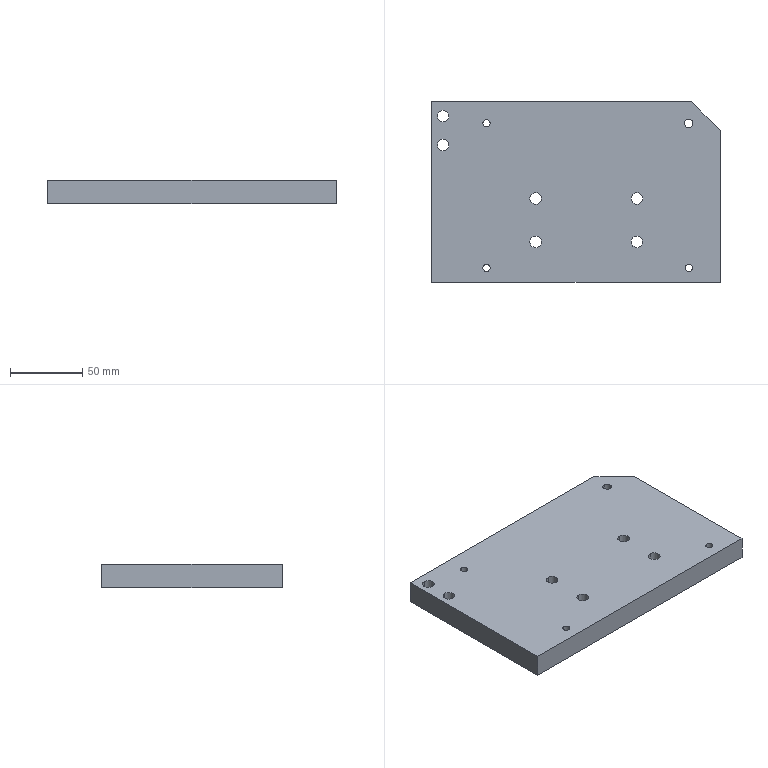Part | STEP file | [15] | 1 solid | 27 faces | box 200 x 125 x 16 mm | volume 390580 mm3 | cylinder 20 | plane 7 | commonest cylinder face diameters 8 x12 5 x6 6 x2
STEP:
#1=CARTESIAN_POINT('',(175.,113.,0.));
#2=VERTEX_POINT('',#1);
#3=CARTESIAN_POINT('',(175.,107.,0.));
#4=VERTEX_POINT('',#3);
#5=CARTESIAN_POINT('',(175.,110.,0.));
#6=DIRECTION('',(0.,0.,1.));
#7=DIRECTION('',(0.,-1.,0.));
#8=AXIS2_PLACEMENT_3D('',#5,#6,#7);
#9=CIRCLE('',#8,3.);
#10=EDGE_CURVE('',#2,#4,#9,.T.);
#11=ORIENTED_EDGE('',*,*,#10,.F.);
#12=CARTESIAN_POINT('',(175.,113.,16.));
#13=VERTEX_POINT('',#12);
#14=CARTESIAN_POINT('',(175.,113.,0.));
#15=DIRECTION('',(0.,0.,1.));
#16=VECTOR('',#15,1000.);
#17=LINE('',#14,#16);
#18=EDGE_CURVE('',#2,#13,#17,.T.);
#19=ORIENTED_EDGE('',*,*,#18,.T.);
#20=CARTESIAN_POINT('',(175.,107.,16.));
#21=VERTEX_POINT('',#20);
#22=CARTESIAN_POINT('',(175.,110.,16.));
#23=DIRECTION('',(0.,0.,-1.));
#24=DIRECTION('',(0.,1.,0.));
#25=AXIS2_PLACEMENT_3D('',#22,#23,#24);
#26=CIRCLE('',#25,3.);
#27=EDGE_CURVE('',#21,#13,#26,.T.);
#28=ORIENTED_EDGE('',*,*,#27,.F.);
#29=CARTESIAN_POINT('',(175.,107.,0.));
#30=DIRECTION('',(0.,0.,1.));
#31=VECTOR('',#30,1000.);
#32=LINE('',#29,#31);
#33=EDGE_CURVE('',#4,#21,#32,.T.);
#34=ORIENTED_EDGE('',*,*,#33,.F.);
#35=EDGE_LOOP('',(#11,#19,#28,#34));
#36=FACE_OUTER_BOUND('',#35,.T.);
#37=CARTESIAN_POINT('',(175.,110.,0.));
#38=DIRECTION('',(0.,0.,1.));
#39=DIRECTION('',(0.,-1.,0.));
#40=AXIS2_PLACEMENT_3D('',#37,#38,#39);
#41=CYLINDRICAL_SURFACE('',#40,3.);
#42=ADVANCED_FACE('',(#36),#41,.F.);
#43=CARTESIAN_POINT('',(35.,112.5,0.));
#44=VERTEX_POINT('',#43);
#45=CARTESIAN_POINT('',(35.,107.5,0.));
#46=VERTEX_POINT('',#45);
#47=CARTESIAN_POINT('',(35.,110.,0.));
#48=DIRECTION('',(0.,0.,1.));
#49=DIRECTION('',(0.,-1.,0.));
#50=AXIS2_PLACEMENT_3D('',#47,#48,#49);
#51=CIRCLE('',#50,2.5);
#52=EDGE_CURVE('',#44,#46,#51,.T.);
#53=ORIENTED_EDGE('',*,*,#52,.F.);
#54=CARTESIAN_POINT('',(35.,112.5,16.));
#55=VERTEX_POINT('',#54);
#56=CARTESIAN_POINT('',(35.,112.5,0.));
#57=DIRECTION('',(0.,0.,1.));
#58=VECTOR('',#57,1000.);
#59=LINE('',#56,#58);
#60=EDGE_CURVE('',#44,#55,#59,.T.);
#61=ORIENTED_EDGE('',*,*,#60,.T.);
#62=CARTESIAN_POINT('',(35.,107.5,16.));
#63=VERTEX_POINT('',#62);
#64=CARTESIAN_POINT('',(35.,110.,16.));
#65=DIRECTION('',(0.,0.,-1.));
#66=DIRECTION('',(0.,1.,0.));
#67=AXIS2_PLACEMENT_3D('',#64,#65,#66);
#68=CIRCLE('',#67,2.5);
#69=EDGE_CURVE('',#63,#55,#68,.T.);
#70=ORIENTED_EDGE('',*,*,#69,.F.);
#71=CARTESIAN_POINT('',(35.,107.5,0.));
#72=DIRECTION('',(0.,0.,1.));
#73=VECTOR('',#72,1000.);
#74=LINE('',#71,#73);
#75=EDGE_CURVE('',#46,#63,#74,.T.);
#76=ORIENTED_EDGE('',*,*,#75,.F.);
#77=EDGE_LOOP('',(#53,#61,#70,#76));
#78=FACE_OUTER_BOUND('',#77,.T.);
#79=CARTESIAN_POINT('',(35.,110.,0.));
#80=DIRECTION('',(0.,0.,1.));
#81=DIRECTION('',(0.,-1.,0.));
#82=AXIS2_PLACEMENT_3D('',#79,#80,#81);
#83=CYLINDRICAL_SURFACE('',#82,2.5);
#84=ADVANCED_FACE('',(#78),#83,.F.);
#85=CARTESIAN_POINT('',(175.,12.5,0.));
#86=VERTEX_POINT('',#85);
#87=CARTESIAN_POINT('',(175.,7.5,0.));
#88=VERTEX_POINT('',#87);
#89=CARTESIAN_POINT('',(175.,10.,0.));
#90=DIRECTION('',(0.,0.,1.));
#91=DIRECTION('',(0.,-1.,0.));
#92=AXIS2_PLACEMENT_3D('',#89,#90,#91);
#93=CIRCLE('',#92,2.5);
#94=EDGE_CURVE('',#86,#88,#93,.T.);
#95=ORIENTED_EDGE('',*,*,#94,.F.);
#96=CARTESIAN_POINT('',(175.,12.5,16.));
#97=VERTEX_POINT('',#96);
#98=CARTESIAN_POINT('',(175.,12.5,0.));
#99=DIRECTION('',(0.,0.,1.));
#100=VECTOR('',#99,1000.);
#101=LINE('',#98,#100);
#102=EDGE_CURVE('',#86,#97,#101,.T.);
#103=ORIENTED_EDGE('',*,*,#102,.T.);
#104=CARTESIAN_POINT('',(175.,7.5,16.));
#105=VERTEX_POINT('',#104);
#106=CARTESIAN_POINT('',(175.,10.,16.));
#107=DIRECTION('',(0.,0.,-1.));
#108=DIRECTION('',(0.,1.,0.));
#109=AXIS2_PLACEMENT_3D('',#106,#107,#108);
#110=CIRCLE('',#109,2.5);
#111=EDGE_CURVE('',#105,#97,#110,.T.);
#112=ORIENTED_EDGE('',*,*,#111,.F.);
#113=CARTESIAN_POINT('',(175.,7.5,0.));
#114=DIRECTION('',(0.,0.,1.));
#115=VECTOR('',#114,1000.);
#116=LINE('',#113,#115);
#117=EDGE_CURVE('',#88,#105,#116,.T.);
#118=ORIENTED_EDGE('',*,*,#117,.F.);
#119=EDGE_LOOP('',(#95,#103,#112,#118));
#120=FACE_OUTER_BOUND('',#119,.T.);
#121=CARTESIAN_POINT('',(175.,10.,0.));
#122=DIRECTION('',(0.,0.,1.));
#123=DIRECTION('',(0.,-1.,0.));
#124=AXIS2_PLACEMENT_3D('',#121,#122,#123);
#125=CYLINDRICAL_SURFACE('',#124,2.5);
#126=ADVANCED_FACE('',(#120),#125,.F.);
#127=CARTESIAN_POINT('',(35.,12.5,0.));
#128=VERTEX_POINT('',#127);
#129=CARTESIAN_POINT('',(35.,7.5,0.));
#130=VERTEX_POINT('',#129);
#131=CARTESIAN_POINT('',(35.,10.,0.));
#132=DIRECTION('',(0.,0.,1.));
#133=DIRECTION('',(0.,-1.,0.));
#134=AXIS2_PLACEMENT_3D('',#131,#132,#133);
#135=CIRCLE('',#134,2.5);
#136=EDGE_CURVE('',#128,#130,#135,.T.);
#137=ORIENTED_EDGE('',*,*,#136,.F.);
#138=CARTESIAN_POINT('',(35.,12.5,16.));
#139=VERTEX_POINT('',#138);
#140=CARTESIAN_POINT('',(35.,12.5,0.));
#141=DIRECTION('',(0.,0.,1.));
#142=VECTOR('',#141,1000.);
#143=LINE('',#140,#142);
#144=EDGE_CURVE('',#128,#139,#143,.T.);
#145=ORIENTED_EDGE('',*,*,#144,.T.);
#146=CARTESIAN_POINT('',(35.,7.5,16.));
#147=VERTEX_POINT('',#146);
#148=CARTESIAN_POINT('',(35.,10.,16.));
#149=DIRECTION('',(0.,0.,-1.));
#150=DIRECTION('',(0.,1.,0.));
#151=AXIS2_PLACEMENT_3D('',#148,#149,#150);
#152=CIRCLE('',#151,2.5);
#153=EDGE_CURVE('',#147,#139,#152,.T.);
#154=ORIENTED_EDGE('',*,*,#153,.F.);
#155=CARTESIAN_POINT('',(35.,7.5,0.));
#156=DIRECTION('',(0.,0.,1.));
#157=VECTOR('',#156,1000.);
#158=LINE('',#155,#157);
#159=EDGE_CURVE('',#130,#147,#158,.T.);
#160=ORIENTED_EDGE('',*,*,#159,.F.);
#161=EDGE_LOOP('',(#137,#145,#154,#160));
#162=FACE_OUTER_BOUND('',#161,.T.);
#163=CARTESIAN_POINT('',(35.,10.,0.));
#164=DIRECTION('',(0.,0.,1.));
#165=DIRECTION('',(0.,-1.,0.));
#166=AXIS2_PLACEMENT_3D('',#163,#164,#165);
#167=CYLINDRICAL_SURFACE('',#166,2.5);
#168=ADVANCED_FACE('',(#162),#167,.F.);
#169=CARTESIAN_POINT('',(5.,119.,0.));
#170=VERTEX_POINT('',#169);
#171=CARTESIAN_POINT('',(5.,111.,0.));
#172=VERTEX_POINT('',#171);
#173=CARTESIAN_POINT('',(5.,115.,0.));
#174=DIRECTION('',(0.,0.,1.));
#175=DIRECTION('',(0.,-1.,0.));
#176=AXIS2_PLACEMENT_3D('',#173,#174,#175);
#177=CIRCLE('',#176,4.);
#178=EDGE_CURVE('',#170,#172,#177,.T.);
#179=ORIENTED_EDGE('',*,*,#178,.F.);
#180=CARTESIAN_POINT('',(5.,119.,16.));
#181=VERTEX_POINT('',#180);
#182=CARTESIAN_POINT('',(5.,119.,0.));
#183=DIRECTION('',(0.,0.,1.));
#184=VECTOR('',#183,1000.);
#185=LINE('',#182,#184);
#186=EDGE_CURVE('',#170,#181,#185,.T.);
#187=ORIENTED_EDGE('',*,*,#186,.T.);
#188=CARTESIAN_POINT('',(5.,111.,16.));
#189=VERTEX_POINT('',#188);
#190=CARTESIAN_POINT('',(5.,115.,16.));
#191=DIRECTION('',(0.,0.,-1.));
#192=DIRECTION('',(0.,1.,0.));
#193=AXIS2_PLACEMENT_3D('',#190,#191,#192);
#194=CIRCLE('',#193,4.);
#195=EDGE_CURVE('',#189,#181,#194,.T.);
#196=ORIENTED_EDGE('',*,*,#195,.F.);
#197=CARTESIAN_POINT('',(5.,111.,0.));
#198=DIRECTION('',(0.,0.,1.));
#199=VECTOR('',#198,1000.);
#200=LINE('',#197,#199);
#201=EDGE_CURVE('',#172,#189,#200,.T.);
#202=ORIENTED_EDGE('',*,*,#201,.F.);
#203=EDGE_LOOP('',(#179,#187,#196,#202));
#204=FACE_OUTER_BOUND('',#203,.T.);
#205=CARTESIAN_POINT('',(5.,115.,0.));
#206=DIRECTION('',(0.,0.,1.));
#207=DIRECTION('',(0.,-1.,0.));
#208=AXIS2_PLACEMENT_3D('',#205,#206,#207);
#209=CYLINDRICAL_SURFACE('',#208,4.);
#210=ADVANCED_FACE('',(#204),#209,.F.);
#211=CARTESIAN_POINT('',(5.,99.,0.));
#212=VERTEX_POINT('',#211);
#213=CARTESIAN_POINT('',(5.,91.,0.));
#214=VERTEX_POINT('',#213);
#215=CARTESIAN_POINT('',(5.,95.,0.));
#216=DIRECTION('',(0.,0.,1.));
#217=DIRECTION('',(0.,-1.,0.));
#218=AXIS2_PLACEMENT_3D('',#215,#216,#217);
#219=CIRCLE('',#218,4.);
#220=EDGE_CURVE('',#212,#214,#219,.T.);
#221=ORIENTED_EDGE('',*,*,#220,.F.);
#222=CARTESIAN_POINT('',(5.,99.,16.));
#223=VERTEX_POINT('',#222);
#224=CARTESIAN_POINT('',(5.,99.,0.));
#225=DIRECTION('',(0.,0.,1.));
#226=VECTOR('',#225,1000.);
#227=LINE('',#224,#226);
#228=EDGE_CURVE('',#212,#223,#227,.T.);
#229=ORIENTED_EDGE('',*,*,#228,.T.);
#230=CARTESIAN_POINT('',(5.,91.,16.));
#231=VERTEX_POINT('',#230);
#232=CARTESIAN_POINT('',(5.,95.,16.));
#233=DIRECTION('',(0.,0.,-1.));
#234=DIRECTION('',(0.,1.,0.));
#235=AXIS2_PLACEMENT_3D('',#232,#233,#234);
#236=CIRCLE('',#235,4.);
#237=EDGE_CURVE('',#231,#223,#236,.T.);
#238=ORIENTED_EDGE('',*,*,#237,.F.);
#239=CARTESIAN_POINT('',(5.,91.,0.));
#240=DIRECTION('',(0.,0.,1.));
#241=VECTOR('',#240,1000.);
#242=LINE('',#239,#241);
#243=EDGE_CURVE('',#214,#231,#242,.T.);
#244=ORIENTED_EDGE('',*,*,#243,.F.);
#245=EDGE_LOOP('',(#221,#229,#238,#244));
#246=FACE_OUTER_BOUND('',#245,.T.);
#247=CARTESIAN_POINT('',(5.,95.,0.));
#248=DIRECTION('',(0.,0.,1.));
#249=DIRECTION('',(0.,-1.,0.));
#250=AXIS2_PLACEMENT_3D('',#247,#248,#249);
#251=CYLINDRICAL_SURFACE('',#250,4.);
#252=ADVANCED_FACE('',(#246),#251,.F.);
#253=CARTESIAN_POINT('',(139.1,32.,0.));
#254=VERTEX_POINT('',#253);
#255=CARTESIAN_POINT('',(139.1,24.,0.));
#256=VERTEX_POINT('',#255);
#257=CARTESIAN_POINT('',(139.1,28.,0.));
#258=DIRECTION('',(0.,0.,1.));
#259=DIRECTION('',(0.,-1.,0.));
#260=AXIS2_PLACEMENT_3D('',#257,#258,#259);
#261=CIRCLE('',#260,4.);
#262=EDGE_CURVE('',#254,#256,#261,.T.);
#263=ORIENTED_EDGE('',*,*,#262,.F.);
#264=CARTESIAN_POINT('',(139.1,32.,16.));
#265=VERTEX_POINT('',#264);
#266=CARTESIAN_POINT('',(139.1,32.,0.));
#267=DIRECTION('',(0.,0.,1.));
#268=VECTOR('',#267,1000.);
#269=LINE('',#266,#268);
#270=EDGE_CURVE('',#254,#265,#269,.T.);
#271=ORIENTED_EDGE('',*,*,#270,.T.);
#272=CARTESIAN_POINT('',(139.1,24.,16.));
#273=VERTEX_POINT('',#272);
#274=CARTESIAN_POINT('',(139.1,28.,16.));
#275=DIRECTION('',(0.,0.,-1.));
#276=DIRECTION('',(0.,1.,0.));
#277=AXIS2_PLACEMENT_3D('',#274,#275,#276);
#278=CIRCLE('',#277,4.);
#279=EDGE_CURVE('',#273,#265,#278,.T.);
#280=ORIENTED_EDGE('',*,*,#279,.F.);
#281=CARTESIAN_POINT('',(139.1,24.,0.));
#282=DIRECTION('',(0.,0.,1.));
#283=VECTOR('',#282,1000.);
#284=LINE('',#281,#283);
#285=EDGE_CURVE('',#256,#273,#284,.T.);
#286=ORIENTED_EDGE('',*,*,#285,.F.);
#287=EDGE_LOOP('',(#263,#271,#280,#286));
#288=FACE_OUTER_BOUND('',#287,.T.);
#289=CARTESIAN_POINT('',(139.1,28.,0.));
#290=DIRECTION('',(0.,0.,1.));
#291=DIRECTION('',(0.,-1.,0.));
#292=AXIS2_PLACEMENT_3D('',#289,#290,#291);
#293=CYLINDRICAL_SURFACE('',#292,4.);
#294=ADVANCED_FACE('',(#288),#293,.F.);
#295=CARTESIAN_POINT('',(139.1,62.,0.));
#296=VERTEX_POINT('',#295);
#297=CARTESIAN_POINT('',(139.1,54.,0.));
#298=VERTEX_POINT('',#297);
#299=CARTESIAN_POINT('',(139.1,58.,0.));
#300=DIRECTION('',(0.,0.,1.));
#301=DIRECTION('',(0.,-1.,0.));
#302=AXIS2_PLACEMENT_3D('',#299,#300,#301);
#303=CIRCLE('',#302,4.);
#304=EDGE_CURVE('',#296,#298,#303,.T.);
#305=ORIENTED_EDGE('',*,*,#304,.F.);
#306=CARTESIAN_POINT('',(139.1,62.,16.));
#307=VERTEX_POINT('',#306);
#308=CARTESIAN_POINT('',(139.1,62.,0.));
#309=DIRECTION('',(0.,0.,1.));
#310=VECTOR('',#309,1000.);
#311=LINE('',#308,#310);
#312=EDGE_CURVE('',#296,#307,#311,.T.);
#313=ORIENTED_EDGE('',*,*,#312,.T.);
#314=CARTESIAN_POINT('',(139.1,54.,16.));
#315=VERTEX_POINT('',#314);
#316=CARTESIAN_POINT('',(139.1,58.,16.));
#317=DIRECTION('',(0.,0.,-1.));
#318=DIRECTION('',(0.,1.,0.));
#319=AXIS2_PLACEMENT_3D('',#316,#317,#318);
#320=CIRCLE('',#319,4.);
#321=EDGE_CURVE('',#315,#307,#320,.T.);
#322=ORIENTED_EDGE('',*,*,#321,.F.);
#323=CARTESIAN_POINT('',(139.1,54.,0.));
#324=DIRECTION('',(0.,0.,1.));
#325=VECTOR('',#324,1000.);
#326=LINE('',#323,#325);
#327=EDGE_CURVE('',#298,#315,#326,.T.);
#328=ORIENTED_EDGE('',*,*,#327,.F.);
#329=EDGE_LOOP('',(#305,#313,#322,#328));
#330=FACE_OUTER_BOUND('',#329,.T.);
#331=CARTESIAN_POINT('',(139.1,58.,0.));
#332=DIRECTION('',(0.,0.,1.));
#333=DIRECTION('',(0.,-1.,0.));
#334=AXIS2_PLACEMENT_3D('',#331,#332,#333);
#335=CYLINDRICAL_SURFACE('',#334,4.);
#336=ADVANCED_FACE('',(#330),#335,.F.);
#337=CARTESIAN_POINT('',(69.1,32.,0.));
#338=VERTEX_POINT('',#337);
#339=CARTESIAN_POINT('',(69.1,24.,0.));
#340=VERTEX_POINT('',#339);
#341=CARTESIAN_POINT('',(69.1,28.,0.));
#342=DIRECTION('',(0.,0.,1.));
#343=DIRECTION('',(0.,-1.,0.));
#344=AXIS2_PLACEMENT_3D('',#341,#342,#343);
#345=CIRCLE('',#344,4.);
#346=EDGE_CURVE('',#338,#340,#345,.T.);
#347=ORIENTED_EDGE('',*,*,#346,.F.);
#348=CARTESIAN_POINT('',(69.1,32.,16.));
#349=VERTEX_POINT('',#348);
#350=CARTESIAN_POINT('',(69.1,32.,0.));
#351=DIRECTION('',(0.,0.,1.));
#352=VECTOR('',#351,1000.);
#353=LINE('',#350,#352);
#354=EDGE_CURVE('',#338,#349,#353,.T.);
#355=ORIENTED_EDGE('',*,*,#354,.T.);
#356=CARTESIAN_POINT('',(69.1,24.,16.));
#357=VERTEX_POINT('',#356);
#358=CARTESIAN_POINT('',(69.1,28.,16.));
#359=DIRECTION('',(0.,0.,-1.));
#360=DIRECTION('',(0.,1.,0.));
#361=AXIS2_PLACEMENT_3D('',#358,#359,#360);
#362=CIRCLE('',#361,4.);
#363=EDGE_CURVE('',#357,#349,#362,.T.);
#364=ORIENTED_EDGE('',*,*,#363,.F.);
#365=CARTESIAN_POINT('',(69.1,24.,0.));
#366=DIRECTION('',(0.,0.,1.));
#367=VECTOR('',#366,1000.);
#368=LINE('',#365,#367);
#369=EDGE_CURVE('',#340,#357,#368,.T.);
#370=ORIENTED_EDGE('',*,*,#369,.F.);
#371=EDGE_LOOP('',(#347,#355,#364,#370));
#372=FACE_OUTER_BOUND('',#371,.T.);
#373=CARTESIAN_POINT('',(69.1,28.,0.));
#374=DIRECTION('',(0.,0.,1.));
#375=DIRECTION('',(0.,-1.,0.));
#376=AXIS2_PLACEMENT_3D('',#373,#374,#375);
#377=CYLINDRICAL_SURFACE('',#376,4.);
#378=ADVANCED_FACE('',(#372),#377,.F.);
#379=CARTESIAN_POINT('',(69.1,62.,0.));
#380=VERTEX_POINT('',#379);
#381=CARTESIAN_POINT('',(69.1,54.,0.));
#382=VERTEX_POINT('',#381);
#383=CARTESIAN_POINT('',(69.1,58.,0.));
#384=DIRECTION('',(0.,0.,1.));
#385=DIRECTION('',(0.,-1.,0.));
#386=AXIS2_PLACEMENT_3D('',#383,#384,#385);
#387=CIRCLE('',#386,4.);
#388=EDGE_CURVE('',#380,#382,#387,.T.);
#389=ORIENTED_EDGE('',*,*,#388,.F.);
#390=CARTESIAN_POINT('',(69.1,62.,16.));
#391=VERTEX_POINT('',#390);
#392=CARTESIAN_POINT('',(69.1,62.,0.));
#393=DIRECTION('',(0.,0.,1.));
#394=VECTOR('',#393,1000.);
#395=LINE('',#392,#394);
#396=EDGE_CURVE('',#380,#391,#395,.T.);
#397=ORIENTED_EDGE('',*,*,#396,.T.);
#398=CARTESIAN_POINT('',(69.1,54.,16.));
#399=VERTEX_POINT('',#398);
#400=CARTESIAN_POINT('',(69.1,58.,16.));
#401=DIRECTION('',(0.,0.,-1.));
#402=DIRECTION('',(0.,1.,0.));
#403=AXIS2_PLACEMENT_3D('',#400,#401,#402);
#404=CIRCLE('',#403,4.);
#405=EDGE_CURVE('',#399,#391,#404,.T.);
#406=ORIENTED_EDGE('',*,*,#405,.F.);
#407=CARTESIAN_POINT('',(69.1,54.,0.));
#408=DIRECTION('',(0.,0.,1.));
#409=VECTOR('',#408,1000.);
#410=LINE('',#407,#409);
#411=EDGE_CURVE('',#382,#399,#410,.T.);
#412=ORIENTED_EDGE('',*,*,#411,.F.);
#413=EDGE_LOOP('',(#389,#397,#406,#412));
#414=FACE_OUTER_BOUND('',#413,.T.);
#415=CARTESIAN_POINT('',(69.1,58.,0.));
#416=DIRECTION('',(0.,0.,1.));
#417=DIRECTION('',(0.,-1.,0.));
#418=AXIS2_PLACEMENT_3D('',#415,#416,#417);
#419=CYLINDRICAL_SURFACE('',#418,4.);
#420=ADVANCED_FACE('',(#414),#419,.F.);
#421=CARTESIAN_POINT('',(175.,110.,0.));
#422=DIRECTION('',(0.,0.,1.));
#423=DIRECTION('',(0.,-1.,0.));
#424=AXIS2_PLACEMENT_3D('',#421,#422,#423);
#425=CIRCLE('',#424,3.);
#426=EDGE_CURVE('',#4,#2,#425,.T.);
#427=ORIENTED_EDGE('',*,*,#426,.T.);
#428=ORIENTED_EDGE('',*,*,#10,.T.);
#429=EDGE_LOOP('',(#427,#428));
#430=FACE_BOUND('',#429,.T.);
#431=CARTESIAN_POINT('',(35.,110.,0.));
#432=DIRECTION('',(0.,0.,1.));
#433=DIRECTION('',(0.,-1.,0.));
#434=AXIS2_PLACEMENT_3D('',#431,#432,#433);
#435=CIRCLE('',#434,2.5);
#436=EDGE_CURVE('',#46,#44,#435,.T.);
#437=ORIENTED_EDGE('',*,*,#436,.T.);
#438=ORIENTED_EDGE('',*,*,#52,.T.);
#439=EDGE_LOOP('',(#437,#438));
#440=FACE_BOUND('',#439,.T.);
#441=CARTESIAN_POINT('',(175.,10.,0.));
#442=DIRECTION('',(0.,0.,1.));
#443=DIRECTION('',(0.,-1.,0.));
#444=AXIS2_PLACEMENT_3D('',#441,#442,#443);
#445=CIRCLE('',#444,2.5);
#446=EDGE_CURVE('',#88,#86,#445,.T.);
#447=ORIENTED_EDGE('',*,*,#446,.T.);
#448=ORIENTED_EDGE('',*,*,#94,.T.);
#449=EDGE_LOOP('',(#447,#448));
#450=FACE_BOUND('',#449,.T.);
#451=CARTESIAN_POINT('',(35.,10.,0.));
#452=DIRECTION('',(0.,0.,1.));
#453=DIRECTION('',(0.,-1.,0.));
#454=AXIS2_PLACEMENT_3D('',#451,#452,#453);
#455=CIRCLE('',#454,2.5);
#456=EDGE_CURVE('',#130,#128,#455,.T.);
#457=ORIENTED_EDGE('',*,*,#456,.T.);
#458=ORIENTED_EDGE('',*,*,#136,.T.);
#459=EDGE_LOOP('',(#457,#458));
#460=FACE_BOUND('',#459,.T.);
#461=CARTESIAN_POINT('',(5.,115.,0.));
#462=DIRECTION('',(0.,0.,1.));
#463=DIRECTION('',(0.,-1.,0.));
#464=AXIS2_PLACEMENT_3D('',#461,#462,#463);
#465=CIRCLE('',#464,4.);
#466=EDGE_CURVE('',#172,#170,#465,.T.);
#467=ORIENTED_EDGE('',*,*,#466,.T.);
#468=ORIENTED_EDGE('',*,*,#178,.T.);
#469=EDGE_LOOP('',(#467,#468));
#470=FACE_BOUND('',#469,.T.);
#471=CARTESIAN_POINT('',(5.,95.,0.));
#472=DIRECTION('',(0.,0.,1.));
#473=DIRECTION('',(0.,-1.,0.));
#474=AXIS2_PLACEMENT_3D('',#471,#472,#473);
#475=CIRCLE('',#474,4.);
#476=EDGE_CURVE('',#214,#212,#475,.T.);
#477=ORIENTED_EDGE('',*,*,#476,.T.);
#478=ORIENTED_EDGE('',*,*,#220,.T.);
#479=EDGE_LOOP('',(#477,#478));
#480=FACE_BOUND('',#479,.T.);
#481=CARTESIAN_POINT('',(139.1,28.,0.));
#482=DIRECTION('',(0.,0.,1.));
#483=DIRECTION('',(0.,-1.,0.));
#484=AXIS2_PLACEMENT_3D('',#481,#482,#483);
#485=CIRCLE('',#484,4.);
#486=EDGE_CURVE('',#256,#254,#485,.T.);
#487=ORIENTED_EDGE('',*,*,#486,.T.);
#488=ORIENTED_EDGE('',*,*,#262,.T.);
#489=EDGE_LOOP('',(#487,#488));
#490=FACE_BOUND('',#489,.T.);
#491=CARTESIAN_POINT('',(139.1,58.,0.));
#492=DIRECTION('',(0.,0.,1.));
#493=DIRECTION('',(0.,-1.,0.));
#494=AXIS2_PLACEMENT_3D('',#491,#492,#493);
#495=CIRCLE('',#494,4.);
#496=EDGE_CURVE('',#298,#296,#495,.T.);
#497=ORIENTED_EDGE('',*,*,#496,.T.);
#498=ORIENTED_EDGE('',*,*,#304,.T.);
#499=EDGE_LOOP('',(#497,#498));
#500=FACE_BOUND('',#499,.T.);
#501=CARTESIAN_POINT('',(69.1,28.,0.));
#502=DIRECTION('',(0.,0.,1.));
#503=DIRECTION('',(0.,-1.,0.));
#504=AXIS2_PLACEMENT_3D('',#501,#502,#503);
#505=CIRCLE('',#504,4.);
#506=EDGE_CURVE('',#340,#338,#505,.T.);
#507=ORIENTED_EDGE('',*,*,#506,.T.);
#508=ORIENTED_EDGE('',*,*,#346,.T.);
#509=EDGE_LOOP('',(#507,#508));
#510=FACE_BOUND('',#509,.T.);
#511=CARTESIAN_POINT('',(69.1,58.,0.));
#512=DIRECTION('',(0.,0.,1.));
#513=DIRECTION('',(0.,-1.,0.));
#514=AXIS2_PLACEMENT_3D('',#511,#512,#513);
#515=CIRCLE('',#514,4.);
#516=EDGE_CURVE('',#382,#380,#515,.T.);
#517=ORIENTED_EDGE('',*,*,#516,.T.);
#518=ORIENTED_EDGE('',*,*,#388,.T.);
#519=EDGE_LOOP('',(#517,#518));
#520=FACE_BOUND('',#519,.T.);
#521=CARTESIAN_POINT('',(177.,125.,0.));
#522=VERTEX_POINT('',#521);
#523=CARTESIAN_POINT('',(-3.,125.,0.));
#524=VERTEX_POINT('',#523);
#525=CARTESIAN_POINT('',(97.,125.,0.));
#526=DIRECTION('',(-1.,0.,0.));
#527=VECTOR('',#526,1000.);
#528=LINE('',#525,#527);
#529=EDGE_CURVE('',#522,#524,#528,.T.);
#530=ORIENTED_EDGE('',*,*,#529,.F.);
#531=CARTESIAN_POINT('',(197.,105.,0.));
#532=VERTEX_POINT('',#531);
#533=CARTESIAN_POINT('',(168.25,133.75,0.));
#534=DIRECTION('',(0.7071,-0.7071,0.));
#535=VECTOR('',#534,1000.);
#536=LINE('',#533,#535);
#537=EDGE_CURVE('',#522,#532,#536,.T.);
#538=ORIENTED_EDGE('',*,*,#537,.T.);
#539=CARTESIAN_POINT('',(197.,0.,0.));
#540=VERTEX_POINT('',#539);
#541=CARTESIAN_POINT('',(197.,62.5,0.));
#542=DIRECTION('',(0.,1.,0.));
#543=VECTOR('',#542,1000.);
#544=LINE('',#541,#543);
#545=EDGE_CURVE('',#540,#532,#544,.T.);
#546=ORIENTED_EDGE('',*,*,#545,.F.);
#547=CARTESIAN_POINT('',(-3.,0.,0.));
#548=VERTEX_POINT('',#547);
#549=CARTESIAN_POINT('',(97.,0.,0.));
#550=DIRECTION('',(1.,0.,0.));
#551=VECTOR('',#550,1000.);
#552=LINE('',#549,#551);
#553=EDGE_CURVE('',#548,#540,#552,.T.);
#554=ORIENTED_EDGE('',*,*,#553,.F.);
#555=CARTESIAN_POINT('',(-3.,62.5,0.));
#556=DIRECTION('',(0.,-1.,0.));
#557=VECTOR('',#556,1000.);
#558=LINE('',#555,#557);
#559=EDGE_CURVE('',#524,#548,#558,.T.);
#560=ORIENTED_EDGE('',*,*,#559,.F.);
#561=EDGE_LOOP('',(#530,#538,#546,#554,#560));
#562=FACE_OUTER_BOUND('',#561,.T.);
#563=CARTESIAN_POINT('',(97.,62.5,0.));
#564=DIRECTION('',(0.,0.,-1.));
#565=DIRECTION('',(0.,1.,0.));
#566=AXIS2_PLACEMENT_3D('',#563,#564,#565);
#567=PLANE('',#566);
#568=ADVANCED_FACE('',(#430,#440,#450,#460,#470,#480,#490,#500,#510,#520,#562),#567,.T.);
#569=CARTESIAN_POINT('',(-3.,125.,16.));
#570=VERTEX_POINT('',#569);
#571=CARTESIAN_POINT('',(-3.,125.,16.));
#572=DIRECTION('',(0.,0.,-1.));
#573=VECTOR('',#572,1000.);
#574=LINE('',#571,#573);
#575=EDGE_CURVE('',#570,#524,#574,.T.);
#576=ORIENTED_EDGE('',*,*,#575,.T.);
#577=ORIENTED_EDGE('',*,*,#559,.T.);
#578=CARTESIAN_POINT('',(-3.,0.,16.));
#579=VERTEX_POINT('',#578);
#580=CARTESIAN_POINT('',(-3.,0.,16.));
#581=DIRECTION('',(0.,0.,-1.));
#582=VECTOR('',#581,1000.);
#583=LINE('',#580,#582);
#584=EDGE_CURVE('',#579,#548,#583,.T.);
#585=ORIENTED_EDGE('',*,*,#584,.F.);
#586=CARTESIAN_POINT('',(-3.,62.5,16.));
#587=DIRECTION('',(0.,1.,0.));
#588=VECTOR('',#587,1000.);
#589=LINE('',#586,#588);
#590=EDGE_CURVE('',#579,#570,#589,.T.);
#591=ORIENTED_EDGE('',*,*,#590,.T.);
#592=EDGE_LOOP('',(#576,#577,#585,#591));
#593=FACE_OUTER_BOUND('',#592,.T.);
#594=CARTESIAN_POINT('',(-3.,62.5,16.));
#595=DIRECTION('',(-1.,0.,0.));
#596=DIRECTION('',(0.,0.,1.));
#597=AXIS2_PLACEMENT_3D('',#594,#595,#596);
#598=PLANE('',#597);
#599=ADVANCED_FACE('',(#593),#598,.T.);
#600=ORIENTED_EDGE('',*,*,#584,.T.);
#601=ORIENTED_EDGE('',*,*,#553,.T.);
#602=CARTESIAN_POINT('',(197.,0.,16.));
#603=VERTEX_POINT('',#602);
#604=CARTESIAN_POINT('',(197.,0.,16.));
#605=DIRECTION('',(0.,0.,-1.));
#606=VECTOR('',#605,1000.);
#607=LINE('',#604,#606);
#608=EDGE_CURVE('',#603,#540,#607,.T.);
#609=ORIENTED_EDGE('',*,*,#608,.F.);
#610=CARTESIAN_POINT('',(97.,0.,16.));
#611=DIRECTION('',(-1.,0.,0.));
#612=VECTOR('',#611,1000.);
#613=LINE('',#610,#612);
#614=EDGE_CURVE('',#603,#579,#613,.T.);
#615=ORIENTED_EDGE('',*,*,#614,.T.);
#616=EDGE_LOOP('',(#600,#601,#609,#615));
#617=FACE_OUTER_BOUND('',#616,.T.);
#618=CARTESIAN_POINT('',(97.,0.,16.));
#619=DIRECTION('',(0.,-1.,0.));
#620=DIRECTION('',(0.,0.,-1.));
#621=AXIS2_PLACEMENT_3D('',#618,#619,#620);
#622=PLANE('',#621);
#623=ADVANCED_FACE('',(#617),#622,.T.);
#624=ORIENTED_EDGE('',*,*,#545,.T.);
#625=CARTESIAN_POINT('',(197.,105.,16.));
#626=VERTEX_POINT('',#625);
#627=CARTESIAN_POINT('',(197.,105.,16.));
#628=DIRECTION('',(0.,0.,1.));
#629=VECTOR('',#628,1000.);
#630=LINE('',#627,#629);
#631=EDGE_CURVE('',#532,#626,#630,.T.);
#632=ORIENTED_EDGE('',*,*,#631,.T.);
#633=CARTESIAN_POINT('',(197.,62.5,16.));
#634=DIRECTION('',(0.,-1.,0.));
#635=VECTOR('',#634,1000.);
#636=LINE('',#633,#635);
#637=EDGE_CURVE('',#626,#603,#636,.T.);
#638=ORIENTED_EDGE('',*,*,#637,.T.);
#639=ORIENTED_EDGE('',*,*,#608,.T.);
#640=EDGE_LOOP('',(#624,#632,#638,#639));
#641=FACE_OUTER_BOUND('',#640,.T.);
#642=CARTESIAN_POINT('',(197.,62.5,16.));
#643=DIRECTION('',(1.,0.,0.));
#644=DIRECTION('',(0.,0.,-1.));
#645=AXIS2_PLACEMENT_3D('',#642,#643,#644);
#646=PLANE('',#645);
#647=ADVANCED_FACE('',(#641),#646,.T.);
#648=ORIENTED_EDGE('',*,*,#27,.T.);
#649=CARTESIAN_POINT('',(175.,110.,16.));
#650=DIRECTION('',(0.,0.,-1.));
#651=DIRECTION('',(0.,1.,0.));
#652=AXIS2_PLACEMENT_3D('',#649,#650,#651);
#653=CIRCLE('',#652,3.);
#654=EDGE_CURVE('',#13,#21,#653,.T.);
#655=ORIENTED_EDGE('',*,*,#654,.T.);
#656=EDGE_LOOP('',(#648,#655));
#657=FACE_BOUND('',#656,.T.);
#658=ORIENTED_EDGE('',*,*,#69,.T.);
#659=CARTESIAN_POINT('',(35.,110.,16.));
#660=DIRECTION('',(0.,0.,-1.));
#661=DIRECTION('',(0.,1.,0.));
#662=AXIS2_PLACEMENT_3D('',#659,#660,#661);
#663=CIRCLE('',#662,2.5);
#664=EDGE_CURVE('',#55,#63,#663,.T.);
#665=ORIENTED_EDGE('',*,*,#664,.T.);
#666=EDGE_LOOP('',(#658,#665));
#667=FACE_BOUND('',#666,.T.);
#668=ORIENTED_EDGE('',*,*,#111,.T.);
#669=CARTESIAN_POINT('',(175.,10.,16.));
#670=DIRECTION('',(0.,0.,-1.));
#671=DIRECTION('',(0.,1.,0.));
#672=AXIS2_PLACEMENT_3D('',#669,#670,#671);
#673=CIRCLE('',#672,2.5);
#674=EDGE_CURVE('',#97,#105,#673,.T.);
#675=ORIENTED_EDGE('',*,*,#674,.T.);
#676=EDGE_LOOP('',(#668,#675));
#677=FACE_BOUND('',#676,.T.);
#678=ORIENTED_EDGE('',*,*,#153,.T.);
#679=CARTESIAN_POINT('',(35.,10.,16.));
#680=DIRECTION('',(0.,0.,-1.));
#681=DIRECTION('',(0.,1.,0.));
#682=AXIS2_PLACEMENT_3D('',#679,#680,#681);
#683=CIRCLE('',#682,2.5);
#684=EDGE_CURVE('',#139,#147,#683,.T.);
#685=ORIENTED_EDGE('',*,*,#684,.T.);
#686=EDGE_LOOP('',(#678,#685));
#687=FACE_BOUND('',#686,.T.);
#688=ORIENTED_EDGE('',*,*,#195,.T.);
#689=CARTESIAN_POINT('',(5.,115.,16.));
#690=DIRECTION('',(0.,0.,-1.));
#691=DIRECTION('',(0.,1.,0.));
#692=AXIS2_PLACEMENT_3D('',#689,#690,#691);
#693=CIRCLE('',#692,4.);
#694=EDGE_CURVE('',#181,#189,#693,.T.);
#695=ORIENTED_EDGE('',*,*,#694,.T.);
#696=EDGE_LOOP('',(#688,#695));
#697=FACE_BOUND('',#696,.T.);
#698=ORIENTED_EDGE('',*,*,#237,.T.);
#699=CARTESIAN_POINT('',(5.,95.,16.));
#700=DIRECTION('',(0.,0.,-1.));
#701=DIRECTION('',(0.,1.,0.));
#702=AXIS2_PLACEMENT_3D('',#699,#700,#701);
#703=CIRCLE('',#702,4.);
#704=EDGE_CURVE('',#223,#231,#703,.T.);
#705=ORIENTED_EDGE('',*,*,#704,.T.);
#706=EDGE_LOOP('',(#698,#705));
#707=FACE_BOUND('',#706,.T.);
#708=ORIENTED_EDGE('',*,*,#279,.T.);
#709=CARTESIAN_POINT('',(139.1,28.,16.));
#710=DIRECTION('',(0.,0.,-1.));
#711=DIRECTION('',(0.,1.,0.));
#712=AXIS2_PLACEMENT_3D('',#709,#710,#711);
#713=CIRCLE('',#712,4.);
#714=EDGE_CURVE('',#265,#273,#713,.T.);
#715=ORIENTED_EDGE('',*,*,#714,.T.);
#716=EDGE_LOOP('',(#708,#715));
#717=FACE_BOUND('',#716,.T.);
#718=ORIENTED_EDGE('',*,*,#321,.T.);
#719=CARTESIAN_POINT('',(139.1,58.,16.));
#720=DIRECTION('',(0.,0.,-1.));
#721=DIRECTION('',(0.,1.,0.));
#722=AXIS2_PLACEMENT_3D('',#719,#720,#721);
#723=CIRCLE('',#722,4.);
#724=EDGE_CURVE('',#307,#315,#723,.T.);
#725=ORIENTED_EDGE('',*,*,#724,.T.);
#726=EDGE_LOOP('',(#718,#725));
#727=FACE_BOUND('',#726,.T.);
#728=ORIENTED_EDGE('',*,*,#363,.T.);
#729=CARTESIAN_POINT('',(69.1,28.,16.));
#730=DIRECTION('',(0.,0.,-1.));
#731=DIRECTION('',(0.,1.,0.));
#732=AXIS2_PLACEMENT_3D('',#729,#730,#731);
#733=CIRCLE('',#732,4.);
#734=EDGE_CURVE('',#349,#357,#733,.T.);
#735=ORIENTED_EDGE('',*,*,#734,.T.);
#736=EDGE_LOOP('',(#728,#735));
#737=FACE_BOUND('',#736,.T.);
#738=ORIENTED_EDGE('',*,*,#405,.T.);
#739=CARTESIAN_POINT('',(69.1,58.,16.));
#740=DIRECTION('',(0.,0.,-1.));
#741=DIRECTION('',(0.,1.,0.));
#742=AXIS2_PLACEMENT_3D('',#739,#740,#741);
#743=CIRCLE('',#742,4.);
#744=EDGE_CURVE('',#391,#399,#743,.T.);
#745=ORIENTED_EDGE('',*,*,#744,.T.);
#746=EDGE_LOOP('',(#738,#745));
#747=FACE_BOUND('',#746,.T.);
#748=ORIENTED_EDGE('',*,*,#637,.F.);
#749=CARTESIAN_POINT('',(177.,125.,16.));
#750=VERTEX_POINT('',#749);
#751=CARTESIAN_POINT('',(168.25,133.75,16.));
#752=DIRECTION('',(-0.7071,0.7071,0.));
#753=VECTOR('',#752,1000.);
#754=LINE('',#751,#753);
#755=EDGE_CURVE('',#626,#750,#754,.T.);
#756=ORIENTED_EDGE('',*,*,#755,.T.);
#757=CARTESIAN_POINT('',(97.,125.,16.));
#758=DIRECTION('',(1.,0.,0.));
#759=VECTOR('',#758,1000.);
#760=LINE('',#757,#759);
#761=EDGE_CURVE('',#570,#750,#760,.T.);
#762=ORIENTED_EDGE('',*,*,#761,.F.);
#763=ORIENTED_EDGE('',*,*,#590,.F.);
#764=ORIENTED_EDGE('',*,*,#614,.F.);
#765=EDGE_LOOP('',(#748,#756,#762,#763,#764));
#766=FACE_OUTER_BOUND('',#765,.T.);
#767=CARTESIAN_POINT('',(97.,62.5,16.));
#768=DIRECTION('',(0.,0.,1.));
#769=DIRECTION('',(0.,-1.,0.));
#770=AXIS2_PLACEMENT_3D('',#767,#768,#769);
#771=PLANE('',#770);
#772=ADVANCED_FACE('',(#657,#667,#677,#687,#697,#707,#717,#727,#737,#747,#766),#771,.T.);
#773=ORIENTED_EDGE('',*,*,#761,.T.);
#774=CARTESIAN_POINT('',(177.,125.,16.));
#775=DIRECTION('',(0.,0.,-1.));
#776=VECTOR('',#775,1000.);
#777=LINE('',#774,#776);
#778=EDGE_CURVE('',#750,#522,#777,.T.);
#779=ORIENTED_EDGE('',*,*,#778,.T.);
#780=ORIENTED_EDGE('',*,*,#529,.T.);
#781=ORIENTED_EDGE('',*,*,#575,.F.);
#782=EDGE_LOOP('',(#773,#779,#780,#781));
#783=FACE_OUTER_BOUND('',#782,.T.);
#784=CARTESIAN_POINT('',(97.,125.,16.));
#785=DIRECTION('',(0.,1.,0.));
#786=DIRECTION('',(0.,0.,1.));
#787=AXIS2_PLACEMENT_3D('',#784,#785,#786);
#788=PLANE('',#787);
#789=ADVANCED_FACE('',(#783),#788,.T.);
#790=ORIENTED_EDGE('',*,*,#396,.F.);
#791=ORIENTED_EDGE('',*,*,#516,.F.);
#792=ORIENTED_EDGE('',*,*,#411,.T.);
#793=ORIENTED_EDGE('',*,*,#744,.F.);
#794=EDGE_LOOP('',(#790,#791,#792,#793));
#795=FACE_OUTER_BOUND('',#794,.T.);
#796=CARTESIAN_POINT('',(69.1,58.,0.));
#797=DIRECTION('',(0.,0.,1.));
#798=DIRECTION('',(0.,-1.,0.));
#799=AXIS2_PLACEMENT_3D('',#796,#797,#798);
#800=CYLINDRICAL_SURFACE('',#799,4.);
#801=ADVANCED_FACE('',(#795),#800,.F.);
#802=ORIENTED_EDGE('',*,*,#354,.F.);
#803=ORIENTED_EDGE('',*,*,#506,.F.);
#804=ORIENTED_EDGE('',*,*,#369,.T.);
#805=ORIENTED_EDGE('',*,*,#734,.F.);
#806=EDGE_LOOP('',(#802,#803,#804,#805));
#807=FACE_OUTER_BOUND('',#806,.T.);
#808=CARTESIAN_POINT('',(69.1,28.,0.));
#809=DIRECTION('',(0.,0.,1.));
#810=DIRECTION('',(0.,-1.,0.));
#811=AXIS2_PLACEMENT_3D('',#808,#809,#810);
#812=CYLINDRICAL_SURFACE('',#811,4.);
#813=ADVANCED_FACE('',(#807),#812,.F.);
#814=ORIENTED_EDGE('',*,*,#312,.F.);
#815=ORIENTED_EDGE('',*,*,#496,.F.);
#816=ORIENTED_EDGE('',*,*,#327,.T.);
#817=ORIENTED_EDGE('',*,*,#724,.F.);
#818=EDGE_LOOP('',(#814,#815,#816,#817));
#819=FACE_OUTER_BOUND('',#818,.T.);
#820=CARTESIAN_POINT('',(139.1,58.,0.));
#821=DIRECTION('',(0.,0.,1.));
#822=DIRECTION('',(0.,-1.,0.));
#823=AXIS2_PLACEMENT_3D('',#820,#821,#822);
#824=CYLINDRICAL_SURFACE('',#823,4.);
#825=ADVANCED_FACE('',(#819),#824,.F.);
#826=ORIENTED_EDGE('',*,*,#270,.F.);
#827=ORIENTED_EDGE('',*,*,#486,.F.);
#828=ORIENTED_EDGE('',*,*,#285,.T.);
#829=ORIENTED_EDGE('',*,*,#714,.F.);
#830=EDGE_LOOP('',(#826,#827,#828,#829));
#831=FACE_OUTER_BOUND('',#830,.T.);
#832=CARTESIAN_POINT('',(139.1,28.,0.));
#833=DIRECTION('',(0.,0.,1.));
#834=DIRECTION('',(0.,-1.,0.));
#835=AXIS2_PLACEMENT_3D('',#832,#833,#834);
#836=CYLINDRICAL_SURFACE('',#835,4.);
#837=ADVANCED_FACE('',(#831),#836,.F.);
#838=ORIENTED_EDGE('',*,*,#228,.F.);
#839=ORIENTED_EDGE('',*,*,#476,.F.);
#840=ORIENTED_EDGE('',*,*,#243,.T.);
#841=ORIENTED_EDGE('',*,*,#704,.F.);
#842=EDGE_LOOP('',(#838,#839,#840,#841));
#843=FACE_OUTER_BOUND('',#842,.T.);
#844=CARTESIAN_POINT('',(5.,95.,0.));
#845=DIRECTION('',(0.,0.,1.));
#846=DIRECTION('',(0.,-1.,0.));
#847=AXIS2_PLACEMENT_3D('',#844,#845,#846);
#848=CYLINDRICAL_SURFACE('',#847,4.);
#849=ADVANCED_FACE('',(#843),#848,.F.);
#850=ORIENTED_EDGE('',*,*,#186,.F.);
#851=ORIENTED_EDGE('',*,*,#466,.F.);
#852=ORIENTED_EDGE('',*,*,#201,.T.);
#853=ORIENTED_EDGE('',*,*,#694,.F.);
#854=EDGE_LOOP('',(#850,#851,#852,#853));
#855=FACE_OUTER_BOUND('',#854,.T.);
#856=CARTESIAN_POINT('',(5.,115.,0.));
#857=DIRECTION('',(0.,0.,1.));
#858=DIRECTION('',(0.,-1.,0.));
#859=AXIS2_PLACEMENT_3D('',#856,#857,#858);
#860=CYLINDRICAL_SURFACE('',#859,4.);
#861=ADVANCED_FACE('',(#855),#860,.F.);
#862=ORIENTED_EDGE('',*,*,#755,.F.);
#863=ORIENTED_EDGE('',*,*,#631,.F.);
#864=ORIENTED_EDGE('',*,*,#537,.F.);
#865=ORIENTED_EDGE('',*,*,#778,.F.);
#866=EDGE_LOOP('',(#862,#863,#864,#865));
#867=FACE_OUTER_BOUND('',#866,.T.);
#868=CARTESIAN_POINT('',(177.,125.,16.));
#869=DIRECTION('',(-0.7071,-0.7071,0.));
#870=DIRECTION('',(0.,0.,-1.));
#871=AXIS2_PLACEMENT_3D('',#868,#869,#870);
#872=PLANE('',#871);
#873=ADVANCED_FACE('',(#867),#872,.F.);
#874=ORIENTED_EDGE('',*,*,#144,.F.);
#875=ORIENTED_EDGE('',*,*,#456,.F.);
#876=ORIENTED_EDGE('',*,*,#159,.T.);
#877=ORIENTED_EDGE('',*,*,#684,.F.);
#878=EDGE_LOOP('',(#874,#875,#876,#877));
#879=FACE_OUTER_BOUND('',#878,.T.);
#880=CARTESIAN_POINT('',(35.,10.,0.));
#881=DIRECTION('',(0.,0.,1.));
#882=DIRECTION('',(0.,-1.,0.));
#883=AXIS2_PLACEMENT_3D('',#880,#881,#882);
#884=CYLINDRICAL_SURFACE('',#883,2.5);
#885=ADVANCED_FACE('',(#879),#884,.F.);
#886=ORIENTED_EDGE('',*,*,#102,.F.);
#887=ORIENTED_EDGE('',*,*,#446,.F.);
#888=ORIENTED_EDGE('',*,*,#117,.T.);
#889=ORIENTED_EDGE('',*,*,#674,.F.);
#890=EDGE_LOOP('',(#886,#887,#888,#889));
#891=FACE_OUTER_BOUND('',#890,.T.);
#892=CARTESIAN_POINT('',(175.,10.,0.));
#893=DIRECTION('',(0.,0.,1.));
#894=DIRECTION('',(0.,-1.,0.));
#895=AXIS2_PLACEMENT_3D('',#892,#893,#894);
#896=CYLINDRICAL_SURFACE('',#895,2.5);
#897=ADVANCED_FACE('',(#891),#896,.F.);
#898=ORIENTED_EDGE('',*,*,#60,.F.);
#899=ORIENTED_EDGE('',*,*,#436,.F.);
#900=ORIENTED_EDGE('',*,*,#75,.T.);
#901=ORIENTED_EDGE('',*,*,#664,.F.);
#902=EDGE_LOOP('',(#898,#899,#900,#901));
#903=FACE_OUTER_BOUND('',#902,.T.);
#904=CARTESIAN_POINT('',(35.,110.,0.));
#905=DIRECTION('',(0.,0.,1.));
#906=DIRECTION('',(0.,-1.,0.));
#907=AXIS2_PLACEMENT_3D('',#904,#905,#906);
#908=CYLINDRICAL_SURFACE('',#907,2.5);
#909=ADVANCED_FACE('',(#903),#908,.F.);
#910=ORIENTED_EDGE('',*,*,#18,.F.);
#911=ORIENTED_EDGE('',*,*,#426,.F.);
#912=ORIENTED_EDGE('',*,*,#33,.T.);
#913=ORIENTED_EDGE('',*,*,#654,.F.);
#914=EDGE_LOOP('',(#910,#911,#912,#913));
#915=FACE_OUTER_BOUND('',#914,.T.);
#916=CARTESIAN_POINT('',(175.,110.,0.));
#917=DIRECTION('',(0.,0.,1.));
#918=DIRECTION('',(0.,-1.,0.));
#919=AXIS2_PLACEMENT_3D('',#916,#917,#918);
#920=CYLINDRICAL_SURFACE('',#919,3.);
#921=ADVANCED_FACE('',(#915),#920,.F.);
#922=CLOSED_SHELL('',(#42,#84,#126,#168,#210,#252,#294,#336,#378,#420,#568,#599,#623,#647,#772,#789,#801,#813,#825,#837,#849,#861,#873,#885,#897,#909,#921));
#923=MANIFOLD_SOLID_BREP('',#922);
#924=CARTESIAN_POINT('',(0.,0.,0.));
#925=DIRECTION('',(0.,0.,1.));
#926=DIRECTION('',(1.,0.,0.));
#927=AXIS2_PLACEMENT_3D('',#924,#925,#926);
#928=(LENGTH_UNIT()NAMED_UNIT(*)SI_UNIT(.MILLI.,.METRE.));
#929=UNCERTAINTY_MEASURE_WITH_UNIT(LENGTH_MEASURE(0.00001),#928,'','');
#930=(NAMED_UNIT(*)PLANE_ANGLE_UNIT()SI_UNIT($,.RADIAN.));
#931=(NAMED_UNIT(*)SI_UNIT($,.STERADIAN.)SOLID_ANGLE_UNIT());
#932=(GEOMETRIC_REPRESENTATION_CONTEXT(3)GLOBAL_UNCERTAINTY_ASSIGNED_CONTEXT((#929))GLOBAL_UNIT_ASSIGNED_CONTEXT((#928,#930,#931))REPRESENTATION_CONTEXT('',''));
#933=ADVANCED_BREP_SHAPE_REPRESENTATION('',(#923,#927),#932);